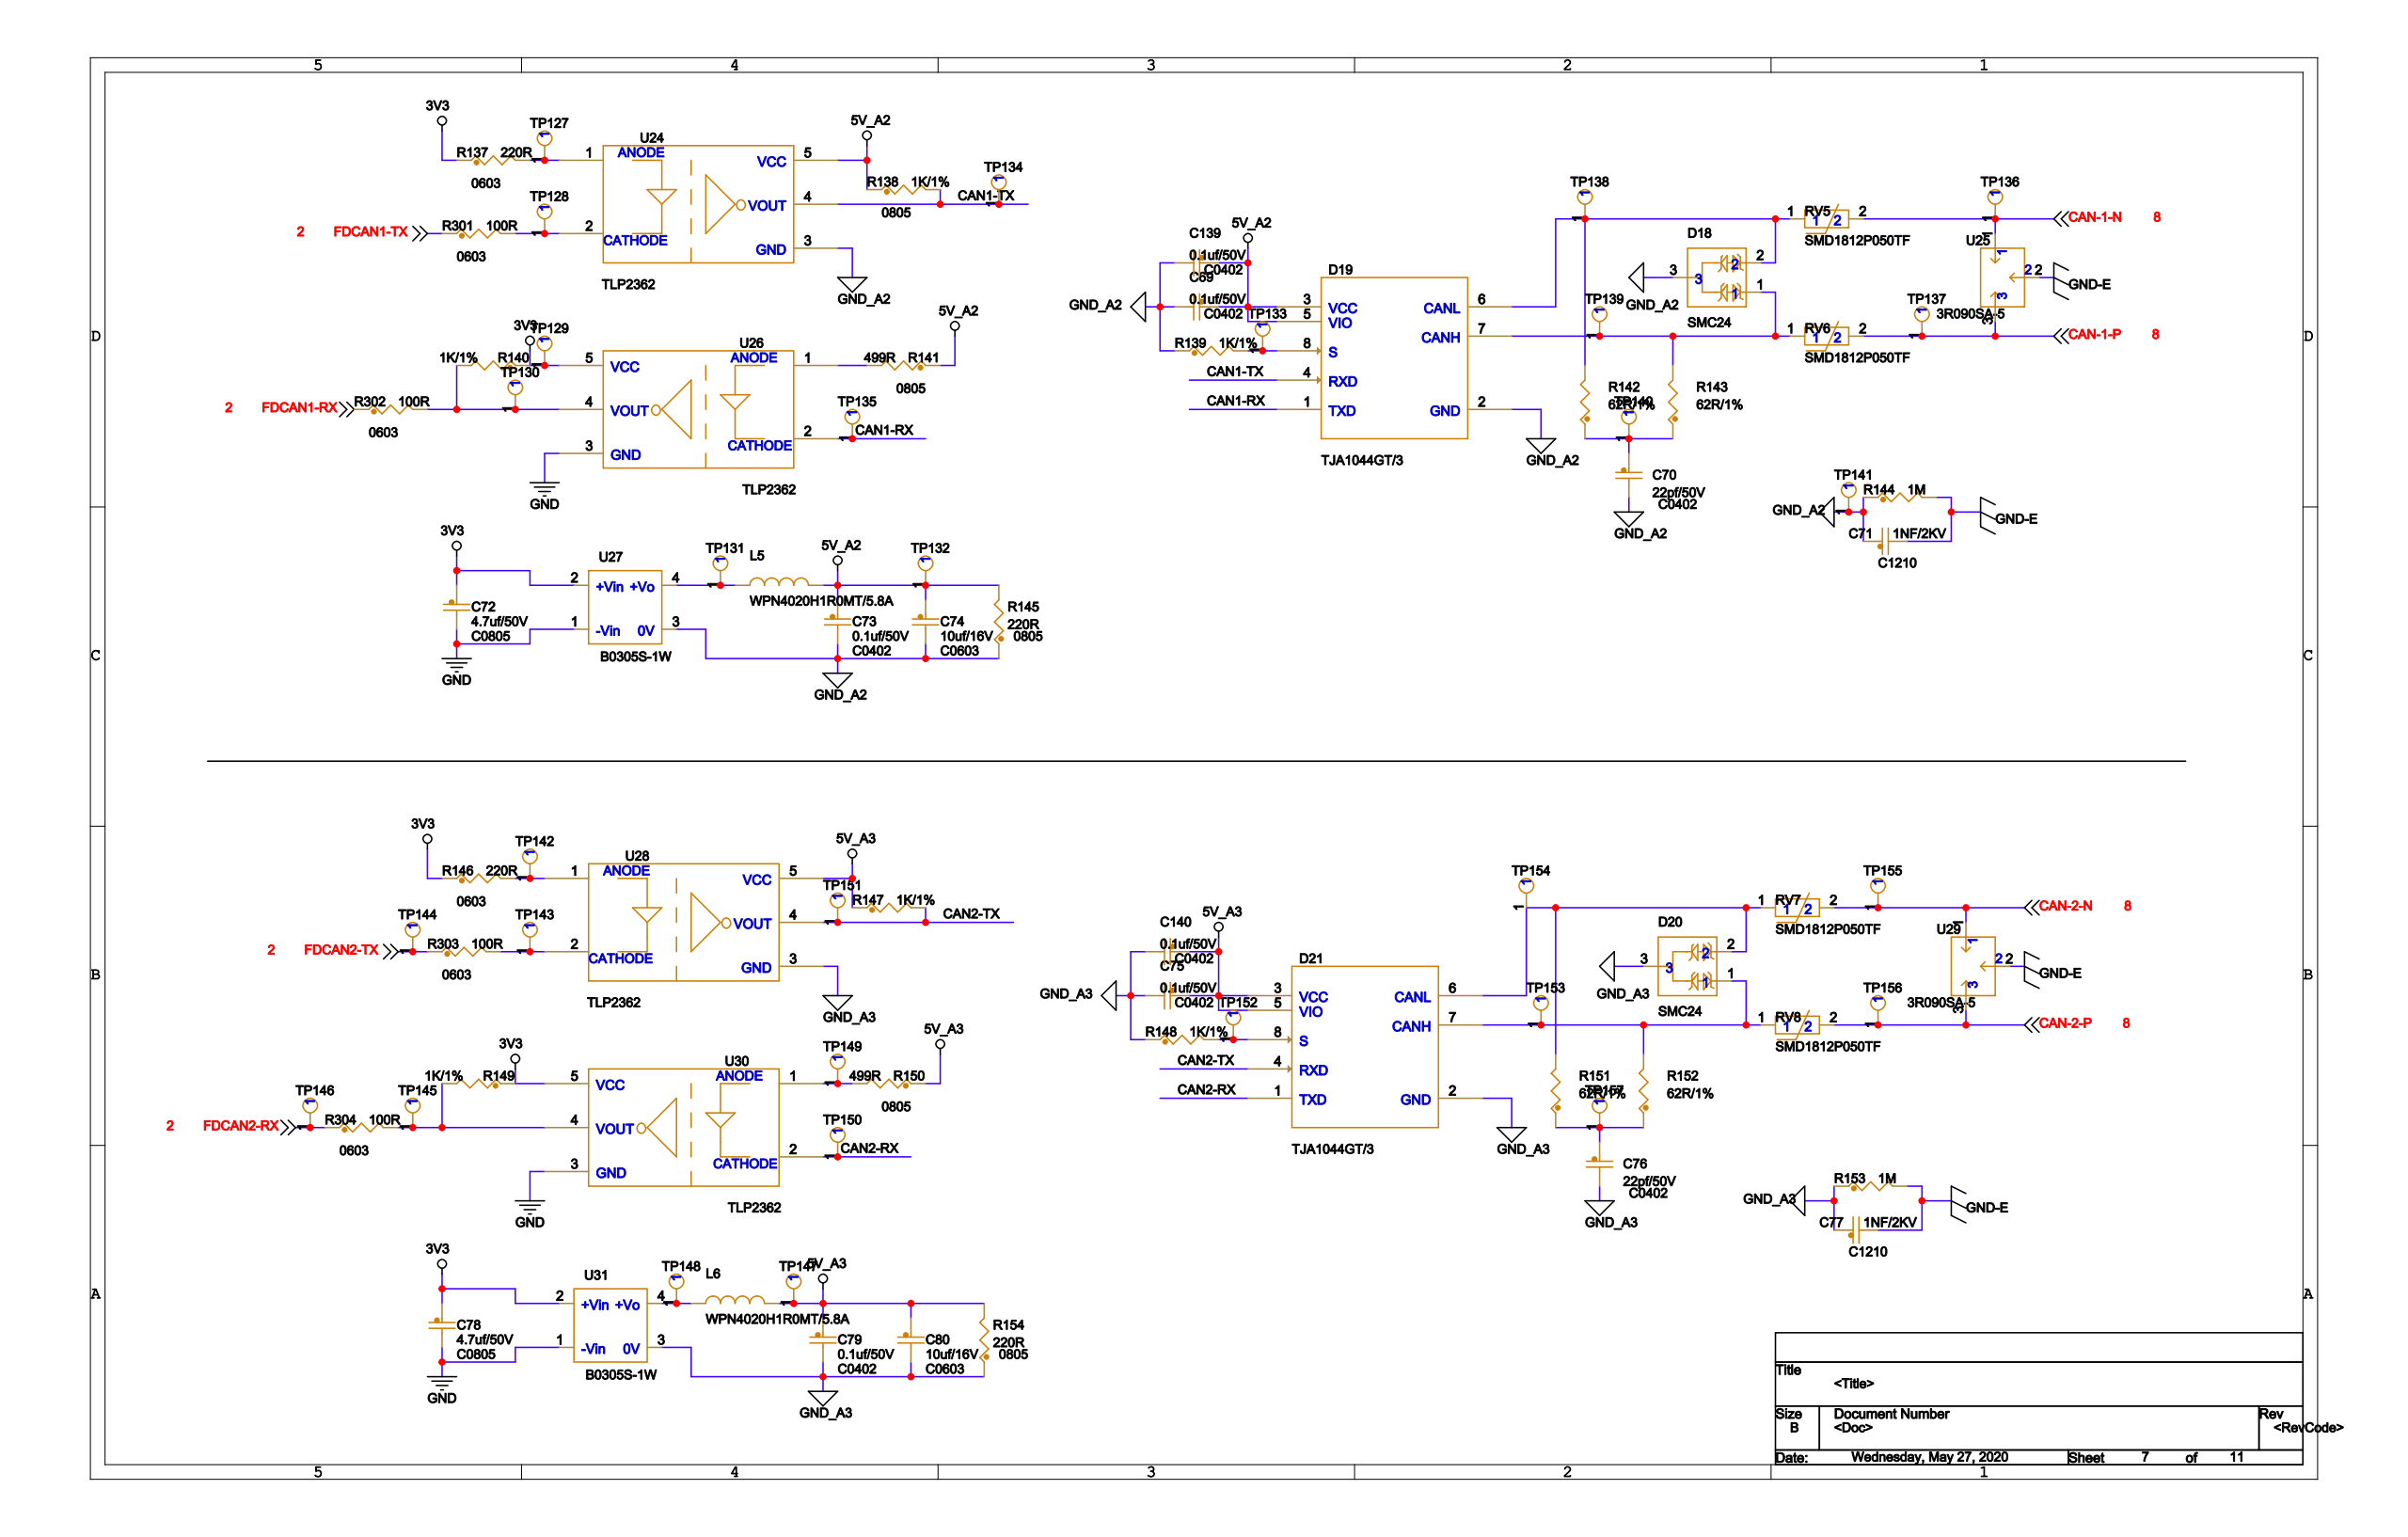Circuit board | Cadence Allegro | 521 parts | 239 nets | one sheet of the schematic
Parts on this sheet (reference | value | footprint):
C69 | 0.1uf/50V | C0402
C70 | 22pf/50V | C0402
C71 | 1NF/2KV | C1210
C72 | 4.7uf/50V | C0805
C73 | 0.1uf/50V | C0402
C74 | 10uf/16V | C0603
C75 | 0.1uf/50V | C0402
C76 | 22pf/50V | C0402
C77 | 1NF/2KV | C1210
C78 | 4.7uf/50V | C0805
C79 | 0.1uf/50V | C0402
C80 | 10uf/16V | C0603
C139 | 0.1uf/50V | C0402
C140 | 0.1uf/50V | C0402
D18 | SMC24 | SOT23
D19 | TJA1044GT/3 | SO8
D20 | SMC24 | SOT23
D21 | TJA1044GT/3 | SO8
L5 | WPN4020H1R0MT/5.8A | SM_IND_4
L6 | WPN4020H1R0MT/5.8A | SM_IND_4
R137 | 220R | 0603
R138 | 1K/1% | 0805
R139 | 1K/1% | 0603
R140 | 1K/1% | 0603
R141 | 499R | 0805
R142 | 62R/1% | 1206
R143 | 62R/1% | 1206
R144 | 1M | 1206
R145 | 220R | 0805
R146 | 220R | 0603
R147 | 1K/1% | 0805
R148 | 1K/1% | 0603
R149 | 1K/1% | 0603
R150 | 499R | 0805
R151 | 62R/1% | 1206
R152 | 62R/1% | 1206
R153 | 1M | 1206
R154 | 220R | 0805
R301 | 100R | 0603
R302 | 100R | 0603
R303 | 100R | 0603
R304 | 100R | 0603
RV5 | SMD1812P050TF | 1812_2
RV6 | SMD1812P050TF | 1812_2
RV7 | SMD1812P050TF | 1812_2
RV8 | SMD1812P050TF | 1812_2
TP127 | TESTPOINT | TESTPOINT-33MIL
TP128 | TESTPOINT | TESTPOINT-33MIL
TP129 | TESTPOINT | TESTPOINT-33MIL
TP130 | TESTPOINT | TESTPOINT-33MIL
TP131 | TESTPOINT | TESTPOINT-33MIL
TP132 | TESTPOINT | TESTPOINT-33MIL
TP133 | TESTPOINT | TESTPOINT-33MIL
TP134 | TESTPOINT | TESTPOINT-33MIL
TP135 | TESTPOINT | TESTPOINT-33MIL
TP136 | TESTPOINT | TESTPOINT-33MIL
TP137 | TESTPOINT | TESTPOINT-33MIL
TP138 | TESTPOINT | TESTPOINT-33MIL
TP139 | TESTPOINT | TESTPOINT-33MIL
TP140 | TESTPOINT | TESTPOINT-33MIL
TP141 | TESTPOINT | TESTPOINT-33MIL
TP142 | TESTPOINT | TESTPOINT-33MIL
TP143 | TESTPOINT | TESTPOINT-33MIL
TP144 | TESTPOINT | TESTPOINT-33MIL
TP145 | TESTPOINT | TESTPOINT-33MIL
TP146 | TESTPOINT | TESTPOINT-33MIL
TP147 | TESTPOINT | TESTPOINT-33MIL
TP148 | TESTPOINT | TESTPOINT-33MIL
TP149 | TESTPOINT | TESTPOINT-33MIL
TP150 | TESTPOINT | TESTPOINT-33MIL
TP151 | TESTPOINT | TESTPOINT-33MIL
TP152 | TESTPOINT | TESTPOINT-33MIL
TP153 | TESTPOINT | TESTPOINT-33MIL
TP154 | TESTPOINT | TESTPOINT-33MIL
TP155 | TESTPOINT | TESTPOINT-33MIL
TP156 | TESTPOINT | TESTPOINT-33MIL
TP157 | TESTPOINT | TESTPOINT-33MIL
U24 | TLP2362 | TLP2362
U25 | 3R090SA-5 | 3R090SA-5
U26 | TLP2362 | TLP2362
U27 | B0305S-1W | B0303S
U28 | TLP2362 | TLP2362
U29 | 3R090SA-5 | 3R090SA-5
U30 | TLP2362 | TLP2362
U31 | B0305S-1W | B0303S
Nets of these parts (net: part-pin ...):
GND: C72-2 C78-2 U26-3 U27-1 U30-3 U31-1
3V3: C72-1 C78-1 R137-1 R140-1 R146-1 R149-1 TP129-1 U26-5 U27-2 U30-5 U31-2
GND-E: C71-2 C77-2 R144-2 R153-2 U25-2 U29-2
N7247638: R137-2 TP127-1 U24-1
N7247642: R301-2 TP128-1 U24-2
N7247810: R140-2 R302-2 TP130-1 U26-4
N7248108: L5-1 TP131-1 U27-4
5V_A2: C69-1 C73-1 C74-1 C139-1 D19-3 D19-5 L5-2 R138-1 R141-1 R145-2 TP132-1 U24-5
N7843129: D19-8 R139-2 TP133-1
CAN1-TX: D19-4 R138-2 TP134-1 U24-4
CAN1-RX: D19-1 TP135-1 U26-2
CAN-1-N: RV5-2 TP136-1 U25-1
CAN-1-P: RV6-2 TP137-1 U25-3
N7247038: D18-2 D19-6 R142-2 RV5-1 TP138-1
N7247046: D18-1 D19-7 R143-2 RV6-1 TP139-1
N7250475: C70-1 R142-1 R143-1 TP140-1
GND_A2: C69-2 C70-2 C71-1 C73-2 C74-2 C139-2 D18-3 D19-2 R139-1 R144-1 R145-1 TP141-1 U24-3 U27-3
N7252703: R146-2 TP142-1 U28-1
N7252707: R303-2 TP143-1 U28-2
FDCAN2-TX: R303-1 TP144-1
N7252749: R149-2 R304-2 TP145-1 U30-4
FDCAN2-RX: R304-1 TP146-1
5V_A3: C75-1 C79-1 C80-1 C140-1 D21-3 D21-5 L6-2 R147-1 R150-1 R154-2 TP147-1 U28-5
N7253075: L6-1 TP148-1 U31-4
N7252789: R150-2 TP149-1 U30-1
CAN2-RX: D21-1 TP150-1 U30-2
CAN2-TX: D21-4 R147-2 TP151-1 U28-4
N7843864: D21-8 R148-2 TP152-1
N7252227: D20-1 D21-7 R152-2 RV8-1 TP153-1
N7252219: D20-2 D21-6 R151-2 RV7-1 TP154-1
CAN-2-N: RV7-2 TP155-1 U29-1
CAN-2-P: RV8-2 TP156-1 U29-3
N7252251: C76-1 R151-1 R152-1 TP157-1
FDCAN1-RX: R302-1
FDCAN1-TX: R301-1
N7247776: R141-2 U26-1
GND_A3: C75-2 C76-2 C77-1 C79-2 C80-2 C140-2 D20-3 D21-2 R148-1 R153-1 R154-1 U28-3 U31-3